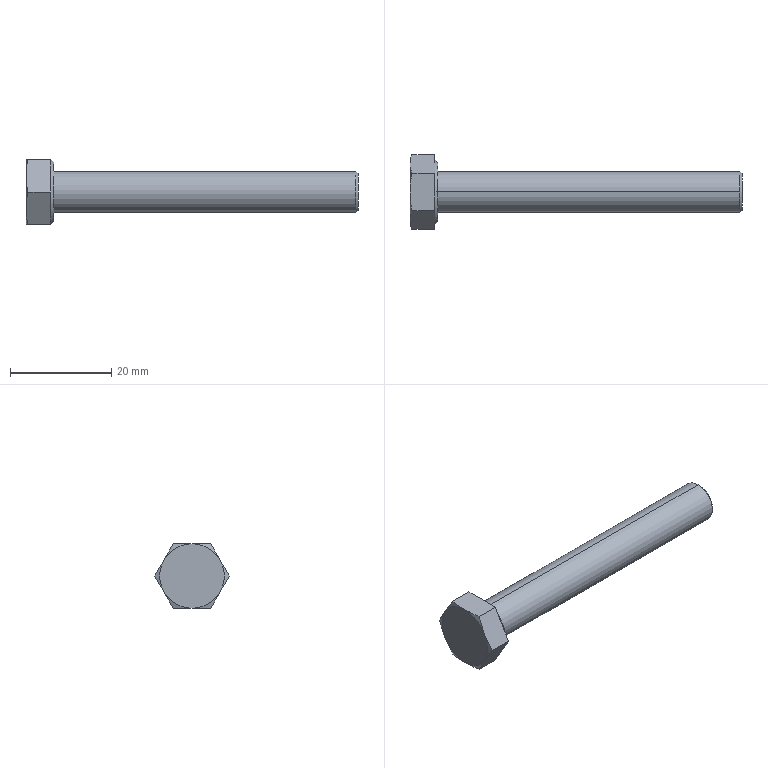Part | STEP file | hexagon head bolts-full thread_gb_GB_FASTENER_BOLT_STBAB A M8X60-N | 1 solid | 27 faces | box 65.45 x 14.699 x 12.73 mm | volume 3764 mm3 | plane 15 | cone 10 | cylinder 2 | commonest cylinder face diameters 8 x2